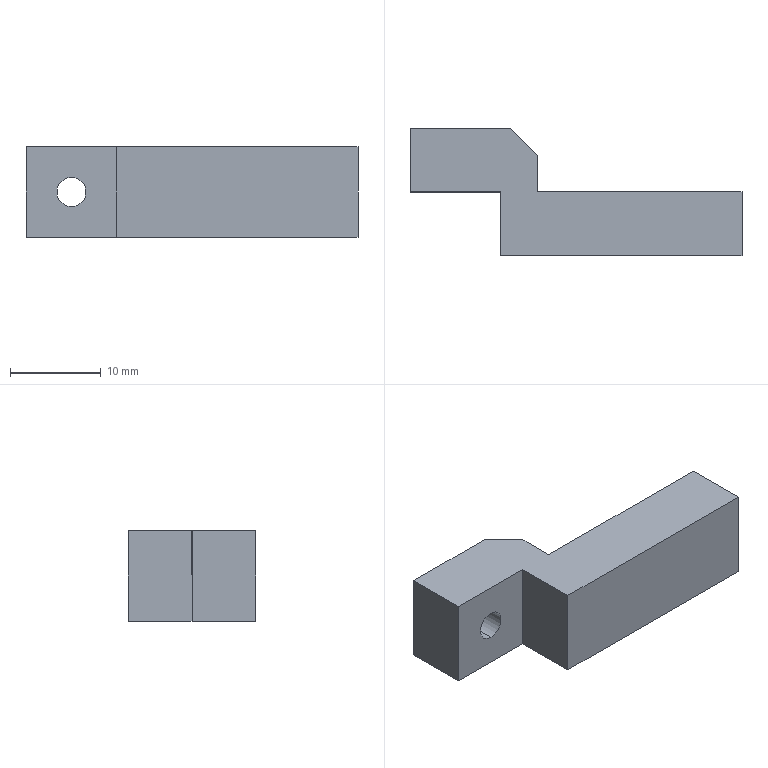Part | NX | features BREP 1 | 1 solid | 16 faces | box 36.5 x 14 x 10 mm | volume 2648 mm3 | plane 12 | cylinder 4 | commonest cylinder face diameters 3.2 x2 6.5 x2
STEP:
#1=CARTESIAN_POINT('',(-13.25,3.6,1.75));
#2=VERTEX_POINT('',#1);
#3=CARTESIAN_POINT('',(-13.25,3.6,8.25));
#4=VERTEX_POINT('',#3);
#5=CARTESIAN_POINT('',(-13.25,3.6,5.));
#6=DIRECTION('',(0.,1.,0.));
#7=DIRECTION('',(0.,0.,1.));
#8=AXIS2_PLACEMENT_3D('',#5,#6,#7);
#9=CIRCLE('',#8,3.25);
#10=EDGE_CURVE('',#2,#4,#9,.T.);
#11=ORIENTED_EDGE('',*,*,#10,.F.);
#12=CARTESIAN_POINT('',(-13.25,7.,1.75));
#13=VERTEX_POINT('',#12);
#14=CARTESIAN_POINT('',(-13.25,7.,1.75));
#15=DIRECTION('',(0.,1.,0.));
#16=VECTOR('',#15,1000.);
#17=LINE('',#14,#16);
#18=EDGE_CURVE('',#13,#2,#17,.F.);
#19=ORIENTED_EDGE('',*,*,#18,.F.);
#20=CARTESIAN_POINT('',(-13.25,7.,8.25));
#21=VERTEX_POINT('',#20);
#22=CARTESIAN_POINT('',(-13.25,7.,5.));
#23=DIRECTION('',(0.,1.,0.));
#24=DIRECTION('',(0.,0.,1.));
#25=AXIS2_PLACEMENT_3D('',#22,#23,#24);
#26=CIRCLE('',#25,3.25);
#27=EDGE_CURVE('',#13,#21,#26,.T.);
#28=ORIENTED_EDGE('',*,*,#27,.T.);
#29=CARTESIAN_POINT('',(-13.25,7.,8.25));
#30=DIRECTION('',(0.,1.,0.));
#31=VECTOR('',#30,1000.);
#32=LINE('',#29,#31);
#33=EDGE_CURVE('',#21,#4,#32,.F.);
#34=ORIENTED_EDGE('',*,*,#33,.T.);
#35=EDGE_LOOP('',(#11,#19,#28,#34));
#36=FACE_BOUND('',#35,.T.);
#37=CARTESIAN_POINT('',(-13.25,7.,5.));
#38=DIRECTION('',(0.,1.,0.));
#39=DIRECTION('',(0.,0.,1.));
#40=AXIS2_PLACEMENT_3D('',#37,#38,#39);
#41=CYLINDRICAL_SURFACE('',#40,3.25);
#42=ADVANCED_FACE('',(#36),#41,.F.);
#43=CARTESIAN_POINT('',(-13.25,0.,3.4));
#44=VERTEX_POINT('',#43);
#45=CARTESIAN_POINT('',(-13.25,0.,6.6));
#46=VERTEX_POINT('',#45);
#47=CARTESIAN_POINT('',(-13.25,0.,5.));
#48=DIRECTION('',(0.,1.,0.));
#49=DIRECTION('',(-1.,0.,0.));
#50=AXIS2_PLACEMENT_3D('',#47,#48,#49);
#51=CIRCLE('',#50,1.6);
#52=EDGE_CURVE('',#44,#46,#51,.T.);
#53=ORIENTED_EDGE('',*,*,#52,.F.);
#54=CARTESIAN_POINT('',(-13.25,3.6,3.4));
#55=VERTEX_POINT('',#54);
#56=CARTESIAN_POINT('',(-13.25,7.,3.4));
#57=DIRECTION('',(0.,1.,0.));
#58=VECTOR('',#57,1000.);
#59=LINE('',#56,#58);
#60=EDGE_CURVE('',#55,#44,#59,.F.);
#61=ORIENTED_EDGE('',*,*,#60,.F.);
#62=CARTESIAN_POINT('',(-13.25,3.6,6.6));
#63=VERTEX_POINT('',#62);
#64=CARTESIAN_POINT('',(-13.25,3.6,5.));
#65=DIRECTION('',(0.,1.,0.));
#66=DIRECTION('',(0.,0.,1.));
#67=AXIS2_PLACEMENT_3D('',#64,#65,#66);
#68=CIRCLE('',#67,1.6);
#69=EDGE_CURVE('',#55,#63,#68,.T.);
#70=ORIENTED_EDGE('',*,*,#69,.T.);
#71=CARTESIAN_POINT('',(-13.25,7.,6.6));
#72=DIRECTION('',(0.,1.,0.));
#73=VECTOR('',#72,1000.);
#74=LINE('',#71,#73);
#75=EDGE_CURVE('',#63,#46,#74,.F.);
#76=ORIENTED_EDGE('',*,*,#75,.T.);
#77=EDGE_LOOP('',(#53,#61,#70,#76));
#78=FACE_BOUND('',#77,.T.);
#79=CARTESIAN_POINT('',(-13.25,7.,5.));
#80=DIRECTION('',(0.,1.,0.));
#81=DIRECTION('',(0.,0.,1.));
#82=AXIS2_PLACEMENT_3D('',#79,#80,#81);
#83=CYLINDRICAL_SURFACE('',#82,1.6);
#84=ADVANCED_FACE('',(#78),#83,.F.);
#85=CARTESIAN_POINT('',(18.25,-7.,0.));
#86=VERTEX_POINT('',#85);
#87=CARTESIAN_POINT('',(18.25,0.,0.));
#88=VERTEX_POINT('',#87);
#89=CARTESIAN_POINT('',(18.25,-7.,0.));
#90=DIRECTION('',(0.,1.,0.));
#91=VECTOR('',#90,1000.);
#92=LINE('',#89,#91);
#93=EDGE_CURVE('',#86,#88,#92,.T.);
#94=ORIENTED_EDGE('',*,*,#93,.T.);
#95=CARTESIAN_POINT('',(18.25,0.,10.));
#96=VERTEX_POINT('',#95);
#97=CARTESIAN_POINT('',(18.25,0.,10.));
#98=DIRECTION('',(0.,0.,1.));
#99=VECTOR('',#98,1000.);
#100=LINE('',#97,#99);
#101=EDGE_CURVE('',#88,#96,#100,.T.);
#102=ORIENTED_EDGE('',*,*,#101,.T.);
#103=CARTESIAN_POINT('',(18.25,-7.,10.));
#104=VERTEX_POINT('',#103);
#105=CARTESIAN_POINT('',(18.25,-7.,10.));
#106=DIRECTION('',(0.,1.,0.));
#107=VECTOR('',#106,1000.);
#108=LINE('',#105,#107);
#109=EDGE_CURVE('',#104,#96,#108,.T.);
#110=ORIENTED_EDGE('',*,*,#109,.F.);
#111=CARTESIAN_POINT('',(18.25,-7.,10.));
#112=DIRECTION('',(0.,0.,-1.));
#113=VECTOR('',#112,1000.);
#114=LINE('',#111,#113);
#115=EDGE_CURVE('',#104,#86,#114,.T.);
#116=ORIENTED_EDGE('',*,*,#115,.T.);
#117=EDGE_LOOP('',(#94,#102,#110,#116));
#118=FACE_BOUND('',#117,.T.);
#119=CARTESIAN_POINT('',(18.25,-7.,10.));
#120=DIRECTION('',(-1.,0.,0.));
#121=DIRECTION('',(0.,0.,1.));
#122=AXIS2_PLACEMENT_3D('',#119,#120,#121);
#123=PLANE('',#122);
#124=ADVANCED_FACE('',(#118),#123,.F.);
#125=CARTESIAN_POINT('',(-7.25,7.,10.));
#126=VERTEX_POINT('',#125);
#127=CARTESIAN_POINT('',(-18.25,7.,10.));
#128=VERTEX_POINT('',#127);
#129=CARTESIAN_POINT('',(-18.25,7.,10.));
#130=DIRECTION('',(-1.,0.,0.));
#131=VECTOR('',#130,1000.);
#132=LINE('',#129,#131);
#133=EDGE_CURVE('',#126,#128,#132,.T.);
#134=ORIENTED_EDGE('',*,*,#133,.F.);
#135=CARTESIAN_POINT('',(-7.25,7.,0.));
#136=VERTEX_POINT('',#135);
#137=CARTESIAN_POINT('',(-7.25,7.,10.));
#138=DIRECTION('',(0.,0.,-1.));
#139=VECTOR('',#138,1000.);
#140=LINE('',#137,#139);
#141=EDGE_CURVE('',#126,#136,#140,.T.);
#142=ORIENTED_EDGE('',*,*,#141,.T.);
#143=CARTESIAN_POINT('',(-18.25,7.,0.));
#144=VERTEX_POINT('',#143);
#145=CARTESIAN_POINT('',(-18.25,7.,0.));
#146=DIRECTION('',(-1.,0.,0.));
#147=VECTOR('',#146,1000.);
#148=LINE('',#145,#147);
#149=EDGE_CURVE('',#136,#144,#148,.T.);
#150=ORIENTED_EDGE('',*,*,#149,.T.);
#151=CARTESIAN_POINT('',(-18.25,7.,10.));
#152=DIRECTION('',(0.,0.,-1.));
#153=VECTOR('',#152,1000.);
#154=LINE('',#151,#153);
#155=EDGE_CURVE('',#128,#144,#154,.T.);
#156=ORIENTED_EDGE('',*,*,#155,.F.);
#157=EDGE_LOOP('',(#134,#142,#150,#156));
#158=FACE_BOUND('',#157,.T.);
#159=CARTESIAN_POINT('',(-13.25,7.,5.));
#160=DIRECTION('',(0.,1.,0.));
#161=DIRECTION('',(0.,0.,1.));
#162=AXIS2_PLACEMENT_3D('',#159,#160,#161);
#163=CIRCLE('',#162,3.25);
#164=EDGE_CURVE('',#21,#13,#163,.T.);
#165=ORIENTED_EDGE('',*,*,#164,.F.);
#166=ORIENTED_EDGE('',*,*,#27,.F.);
#167=EDGE_LOOP('',(#165,#166));
#168=FACE_BOUND('',#167,.T.);
#169=CARTESIAN_POINT('',(-18.25,7.,10.));
#170=DIRECTION('',(0.,-1.,0.));
#171=DIRECTION('',(0.,0.,-1.));
#172=AXIS2_PLACEMENT_3D('',#169,#170,#171);
#173=PLANE('',#172);
#174=ADVANCED_FACE('',(#158,#168),#173,.F.);
#175=CARTESIAN_POINT('',(-18.25,0.,0.));
#176=VERTEX_POINT('',#175);
#177=CARTESIAN_POINT('',(-18.25,-7.,0.));
#178=DIRECTION('',(0.,-1.,0.));
#179=VECTOR('',#178,1000.);
#180=LINE('',#177,#179);
#181=EDGE_CURVE('',#144,#176,#180,.T.);
#182=ORIENTED_EDGE('',*,*,#181,.T.);
#183=CARTESIAN_POINT('',(-18.25,0.,10.));
#184=VERTEX_POINT('',#183);
#185=CARTESIAN_POINT('',(-18.25,0.,10.));
#186=DIRECTION('',(0.,0.,1.));
#187=VECTOR('',#186,1000.);
#188=LINE('',#185,#187);
#189=EDGE_CURVE('',#176,#184,#188,.T.);
#190=ORIENTED_EDGE('',*,*,#189,.T.);
#191=CARTESIAN_POINT('',(-18.25,-7.,10.));
#192=DIRECTION('',(0.,-1.,0.));
#193=VECTOR('',#192,1000.);
#194=LINE('',#191,#193);
#195=EDGE_CURVE('',#128,#184,#194,.T.);
#196=ORIENTED_EDGE('',*,*,#195,.F.);
#197=ORIENTED_EDGE('',*,*,#155,.T.);
#198=EDGE_LOOP('',(#182,#190,#196,#197));
#199=FACE_BOUND('',#198,.T.);
#200=CARTESIAN_POINT('',(-18.25,-7.,10.));
#201=DIRECTION('',(1.,0.,0.));
#202=DIRECTION('',(0.,1.,0.));
#203=AXIS2_PLACEMENT_3D('',#200,#201,#202);
#204=PLANE('',#203);
#205=ADVANCED_FACE('',(#199),#204,.F.);
#206=CARTESIAN_POINT('',(-8.25,-7.,10.));
#207=VERTEX_POINT('',#206);
#208=CARTESIAN_POINT('',(-18.25,-7.,10.));
#209=DIRECTION('',(1.,0.,0.));
#210=VECTOR('',#209,1000.);
#211=LINE('',#208,#210);
#212=EDGE_CURVE('',#207,#104,#211,.T.);
#213=ORIENTED_EDGE('',*,*,#212,.F.);
#214=CARTESIAN_POINT('',(-8.25,-7.,0.));
#215=VERTEX_POINT('',#214);
#216=CARTESIAN_POINT('',(-8.25,-7.,10.));
#217=DIRECTION('',(0.,0.,-1.));
#218=VECTOR('',#217,1000.);
#219=LINE('',#216,#218);
#220=EDGE_CURVE('',#207,#215,#219,.T.);
#221=ORIENTED_EDGE('',*,*,#220,.T.);
#222=CARTESIAN_POINT('',(-18.25,-7.,0.));
#223=DIRECTION('',(1.,0.,0.));
#224=VECTOR('',#223,1000.);
#225=LINE('',#222,#224);
#226=EDGE_CURVE('',#215,#86,#225,.T.);
#227=ORIENTED_EDGE('',*,*,#226,.T.);
#228=ORIENTED_EDGE('',*,*,#115,.F.);
#229=EDGE_LOOP('',(#213,#221,#227,#228));
#230=FACE_BOUND('',#229,.T.);
#231=CARTESIAN_POINT('',(-18.25,-7.,10.));
#232=DIRECTION('',(0.,1.,0.));
#233=DIRECTION('',(1.,0.,0.));
#234=AXIS2_PLACEMENT_3D('',#231,#232,#233);
#235=PLANE('',#234);
#236=ADVANCED_FACE('',(#230),#235,.F.);
#237=CARTESIAN_POINT('',(-4.25,0.,10.));
#238=VERTEX_POINT('',#237);
#239=CARTESIAN_POINT('',(-4.25,4.,10.));
#240=VERTEX_POINT('',#239);
#241=CARTESIAN_POINT('',(-4.25,10.855,10.));
#242=DIRECTION('',(0.,1.,0.));
#243=VECTOR('',#242,1000.);
#244=LINE('',#241,#243);
#245=EDGE_CURVE('',#238,#240,#244,.T.);
#246=ORIENTED_EDGE('',*,*,#245,.T.);
#247=CARTESIAN_POINT('',(-7.25,7.,10.));
#248=DIRECTION('',(-0.7071,0.7071,0.));
#249=VECTOR('',#248,1000.);
#250=LINE('',#247,#249);
#251=EDGE_CURVE('',#240,#126,#250,.T.);
#252=ORIENTED_EDGE('',*,*,#251,.T.);
#253=ORIENTED_EDGE('',*,*,#133,.T.);
#254=ORIENTED_EDGE('',*,*,#195,.T.);
#255=CARTESIAN_POINT('',(-8.25,0.,10.));
#256=VERTEX_POINT('',#255);
#257=CARTESIAN_POINT('',(-8.25,0.,10.));
#258=DIRECTION('',(1.,0.,0.));
#259=VECTOR('',#258,1000.);
#260=LINE('',#257,#259);
#261=EDGE_CURVE('',#184,#256,#260,.T.);
#262=ORIENTED_EDGE('',*,*,#261,.T.);
#263=CARTESIAN_POINT('',(-8.25,0.,10.));
#264=DIRECTION('',(0.,-1.,0.));
#265=VECTOR('',#264,1000.);
#266=LINE('',#263,#265);
#267=EDGE_CURVE('',#256,#207,#266,.T.);
#268=ORIENTED_EDGE('',*,*,#267,.T.);
#269=ORIENTED_EDGE('',*,*,#212,.T.);
#270=ORIENTED_EDGE('',*,*,#109,.T.);
#271=CARTESIAN_POINT('',(-4.25,0.,10.));
#272=DIRECTION('',(-1.,0.,0.));
#273=VECTOR('',#272,1000.);
#274=LINE('',#271,#273);
#275=EDGE_CURVE('',#96,#238,#274,.T.);
#276=ORIENTED_EDGE('',*,*,#275,.T.);
#277=EDGE_LOOP('',(#246,#252,#253,#254,#262,#268,#269,#270,#276));
#278=FACE_BOUND('',#277,.T.);
#279=CARTESIAN_POINT('',(0.,0.,10.));
#280=DIRECTION('',(0.,0.,-1.));
#281=DIRECTION('',(0.,-1.,0.));
#282=AXIS2_PLACEMENT_3D('',#279,#280,#281);
#283=PLANE('',#282);
#284=ADVANCED_FACE('',(#278),#283,.F.);
#285=ORIENTED_EDGE('',*,*,#149,.F.);
#286=CARTESIAN_POINT('',(-4.25,4.,0.));
#287=VERTEX_POINT('',#286);
#288=CARTESIAN_POINT('',(-0.125,-0.125,0.));
#289=DIRECTION('',(0.7071,-0.7071,0.));
#290=VECTOR('',#289,1000.);
#291=LINE('',#288,#290);
#292=EDGE_CURVE('',#136,#287,#291,.T.);
#293=ORIENTED_EDGE('',*,*,#292,.T.);
#294=CARTESIAN_POINT('',(-4.25,0.,0.));
#295=VERTEX_POINT('',#294);
#296=CARTESIAN_POINT('',(-4.25,10.855,0.));
#297=DIRECTION('',(0.,1.,0.));
#298=VECTOR('',#297,1000.);
#299=LINE('',#296,#298);
#300=EDGE_CURVE('',#295,#287,#299,.T.);
#301=ORIENTED_EDGE('',*,*,#300,.F.);
#302=CARTESIAN_POINT('',(0.,0.,0.));
#303=DIRECTION('',(-1.,0.,0.));
#304=VECTOR('',#303,1000.);
#305=LINE('',#302,#304);
#306=EDGE_CURVE('',#88,#295,#305,.T.);
#307=ORIENTED_EDGE('',*,*,#306,.F.);
#308=ORIENTED_EDGE('',*,*,#93,.F.);
#309=ORIENTED_EDGE('',*,*,#226,.F.);
#310=CARTESIAN_POINT('',(-8.25,0.,0.));
#311=VERTEX_POINT('',#310);
#312=CARTESIAN_POINT('',(-8.25,0.,0.));
#313=DIRECTION('',(0.,-1.,0.));
#314=VECTOR('',#313,1000.);
#315=LINE('',#312,#314);
#316=EDGE_CURVE('',#311,#215,#315,.T.);
#317=ORIENTED_EDGE('',*,*,#316,.F.);
#318=CARTESIAN_POINT('',(0.,0.,0.));
#319=DIRECTION('',(1.,0.,0.));
#320=VECTOR('',#319,1000.);
#321=LINE('',#318,#320);
#322=EDGE_CURVE('',#176,#311,#321,.T.);
#323=ORIENTED_EDGE('',*,*,#322,.F.);
#324=ORIENTED_EDGE('',*,*,#181,.F.);
#325=EDGE_LOOP('',(#285,#293,#301,#307,#308,#309,#317,#323,#324));
#326=FACE_BOUND('',#325,.T.);
#327=CARTESIAN_POINT('',(0.,0.,0.));
#328=DIRECTION('',(0.,0.,-1.));
#329=DIRECTION('',(0.,-1.,0.));
#330=AXIS2_PLACEMENT_3D('',#327,#328,#329);
#331=PLANE('',#330);
#332=ADVANCED_FACE('',(#326),#331,.T.);
#333=ORIENTED_EDGE('',*,*,#267,.F.);
#334=CARTESIAN_POINT('',(-8.25,0.,10.));
#335=DIRECTION('',(0.,0.,-1.));
#336=VECTOR('',#335,1000.);
#337=LINE('',#334,#336);
#338=EDGE_CURVE('',#256,#311,#337,.T.);
#339=ORIENTED_EDGE('',*,*,#338,.T.);
#340=ORIENTED_EDGE('',*,*,#316,.T.);
#341=ORIENTED_EDGE('',*,*,#220,.F.);
#342=EDGE_LOOP('',(#333,#339,#340,#341));
#343=FACE_BOUND('',#342,.T.);
#344=CARTESIAN_POINT('',(-8.25,0.,10.));
#345=DIRECTION('',(1.,0.,0.));
#346=DIRECTION('',(0.,-1.,0.));
#347=AXIS2_PLACEMENT_3D('',#344,#345,#346);
#348=PLANE('',#347);
#349=ADVANCED_FACE('',(#343),#348,.F.);
#350=ORIENTED_EDGE('',*,*,#322,.T.);
#351=ORIENTED_EDGE('',*,*,#338,.F.);
#352=ORIENTED_EDGE('',*,*,#261,.F.);
#353=ORIENTED_EDGE('',*,*,#189,.F.);
#354=EDGE_LOOP('',(#350,#351,#352,#353));
#355=FACE_BOUND('',#354,.T.);
#356=CARTESIAN_POINT('',(-13.25,0.,5.));
#357=DIRECTION('',(0.,1.,0.));
#358=DIRECTION('',(-1.,0.,0.));
#359=AXIS2_PLACEMENT_3D('',#356,#357,#358);
#360=CIRCLE('',#359,1.6);
#361=EDGE_CURVE('',#46,#44,#360,.T.);
#362=ORIENTED_EDGE('',*,*,#361,.T.);
#363=ORIENTED_EDGE('',*,*,#52,.T.);
#364=EDGE_LOOP('',(#362,#363));
#365=FACE_BOUND('',#364,.T.);
#366=CARTESIAN_POINT('',(-8.25,0.,10.));
#367=DIRECTION('',(0.,1.,0.));
#368=DIRECTION('',(1.,0.,0.));
#369=AXIS2_PLACEMENT_3D('',#366,#367,#368);
#370=PLANE('',#369);
#371=ADVANCED_FACE('',(#355,#365),#370,.F.);
#372=ORIENTED_EDGE('',*,*,#300,.T.);
#373=CARTESIAN_POINT('',(-4.25,4.,10.));
#374=DIRECTION('',(0.,0.,1.));
#375=VECTOR('',#374,1000.);
#376=LINE('',#373,#375);
#377=EDGE_CURVE('',#287,#240,#376,.T.);
#378=ORIENTED_EDGE('',*,*,#377,.T.);
#379=ORIENTED_EDGE('',*,*,#245,.F.);
#380=CARTESIAN_POINT('',(-4.25,0.,10.));
#381=DIRECTION('',(0.,0.,-1.));
#382=VECTOR('',#381,1000.);
#383=LINE('',#380,#382);
#384=EDGE_CURVE('',#238,#295,#383,.T.);
#385=ORIENTED_EDGE('',*,*,#384,.T.);
#386=EDGE_LOOP('',(#372,#378,#379,#385));
#387=FACE_BOUND('',#386,.T.);
#388=CARTESIAN_POINT('',(-4.25,10.855,10.));
#389=DIRECTION('',(-1.,0.,0.));
#390=DIRECTION('',(0.,0.,1.));
#391=AXIS2_PLACEMENT_3D('',#388,#389,#390);
#392=PLANE('',#391);
#393=ADVANCED_FACE('',(#387),#392,.F.);
#394=ORIENTED_EDGE('',*,*,#306,.T.);
#395=ORIENTED_EDGE('',*,*,#384,.F.);
#396=ORIENTED_EDGE('',*,*,#275,.F.);
#397=ORIENTED_EDGE('',*,*,#101,.F.);
#398=EDGE_LOOP('',(#394,#395,#396,#397));
#399=FACE_BOUND('',#398,.T.);
#400=CARTESIAN_POINT('',(-4.25,0.,10.));
#401=DIRECTION('',(0.,-1.,0.));
#402=DIRECTION('',(-1.,0.,0.));
#403=AXIS2_PLACEMENT_3D('',#400,#401,#402);
#404=PLANE('',#403);
#405=ADVANCED_FACE('',(#399),#404,.F.);
#406=ORIENTED_EDGE('',*,*,#60,.T.);
#407=ORIENTED_EDGE('',*,*,#361,.F.);
#408=ORIENTED_EDGE('',*,*,#75,.F.);
#409=CARTESIAN_POINT('',(-13.25,3.6,5.));
#410=DIRECTION('',(0.,1.,0.));
#411=DIRECTION('',(0.,0.,1.));
#412=AXIS2_PLACEMENT_3D('',#409,#410,#411);
#413=CIRCLE('',#412,1.6);
#414=EDGE_CURVE('',#63,#55,#413,.T.);
#415=ORIENTED_EDGE('',*,*,#414,.T.);
#416=EDGE_LOOP('',(#406,#407,#408,#415));
#417=FACE_BOUND('',#416,.T.);
#418=CARTESIAN_POINT('',(-13.25,7.,5.));
#419=DIRECTION('',(0.,1.,0.));
#420=DIRECTION('',(0.,0.,1.));
#421=AXIS2_PLACEMENT_3D('',#418,#419,#420);
#422=CYLINDRICAL_SURFACE('',#421,1.6);
#423=ADVANCED_FACE('',(#417),#422,.F.);
#424=CARTESIAN_POINT('',(-13.25,3.6,5.));
#425=DIRECTION('',(0.,1.,0.));
#426=DIRECTION('',(0.,0.,1.));
#427=AXIS2_PLACEMENT_3D('',#424,#425,#426);
#428=CIRCLE('',#427,3.25);
#429=EDGE_CURVE('',#4,#2,#428,.T.);
#430=ORIENTED_EDGE('',*,*,#429,.T.);
#431=ORIENTED_EDGE('',*,*,#10,.T.);
#432=EDGE_LOOP('',(#430,#431));
#433=FACE_BOUND('',#432,.T.);
#434=ORIENTED_EDGE('',*,*,#414,.F.);
#435=ORIENTED_EDGE('',*,*,#69,.F.);
#436=EDGE_LOOP('',(#434,#435));
#437=FACE_BOUND('',#436,.T.);
#438=CARTESIAN_POINT('',(-11.65,3.6,5.));
#439=DIRECTION('',(0.,-1.,0.));
#440=DIRECTION('',(0.,0.,-1.));
#441=AXIS2_PLACEMENT_3D('',#438,#439,#440);
#442=PLANE('',#441);
#443=ADVANCED_FACE('',(#433,#437),#442,.F.);
#444=ORIENTED_EDGE('',*,*,#18,.T.);
#445=ORIENTED_EDGE('',*,*,#429,.F.);
#446=ORIENTED_EDGE('',*,*,#33,.F.);
#447=ORIENTED_EDGE('',*,*,#164,.T.);
#448=EDGE_LOOP('',(#444,#445,#446,#447));
#449=FACE_BOUND('',#448,.T.);
#450=CARTESIAN_POINT('',(-13.25,7.,5.));
#451=DIRECTION('',(0.,1.,0.));
#452=DIRECTION('',(0.,0.,1.));
#453=AXIS2_PLACEMENT_3D('',#450,#451,#452);
#454=CYLINDRICAL_SURFACE('',#453,3.25);
#455=ADVANCED_FACE('',(#449),#454,.F.);
#456=ORIENTED_EDGE('',*,*,#251,.F.);
#457=ORIENTED_EDGE('',*,*,#377,.F.);
#458=ORIENTED_EDGE('',*,*,#292,.F.);
#459=ORIENTED_EDGE('',*,*,#141,.F.);
#460=EDGE_LOOP('',(#456,#457,#458,#459));
#461=FACE_BOUND('',#460,.T.);
#462=CARTESIAN_POINT('',(-7.25,7.,10.));
#463=DIRECTION('',(-0.7071,-0.7071,0.));
#464=DIRECTION('',(-0.7071,0.7071,0.));
#465=AXIS2_PLACEMENT_3D('',#462,#463,#464);
#466=PLANE('',#465);
#467=ADVANCED_FACE('',(#461),#466,.F.);
#468=CLOSED_SHELL('',(#42,#84,#124,#174,#205,#236,#284,#332,#349,#371,#393,#405,#423,#443,#455,#467));
#469=MANIFOLD_SOLID_BREP('',#468);
#470=(LENGTH_UNIT()NAMED_UNIT(*)SI_UNIT(.MILLI.,.METRE.));
#471=UNCERTAINTY_MEASURE_WITH_UNIT(LENGTH_MEASURE(0.00001),#470,'','');
#472=(NAMED_UNIT(*)PLANE_ANGLE_UNIT()SI_UNIT($,.RADIAN.));
#473=(NAMED_UNIT(*)SI_UNIT($,.STERADIAN.)SOLID_ANGLE_UNIT());
#474=(GEOMETRIC_REPRESENTATION_CONTEXT(3)GLOBAL_UNCERTAINTY_ASSIGNED_CONTEXT((#471))GLOBAL_UNIT_ASSIGNED_CONTEXT((#470,#472,#473))REPRESENTATION_CONTEXT('',''));
#475=ADVANCED_BREP_SHAPE_REPRESENTATION('',(#469),#474);